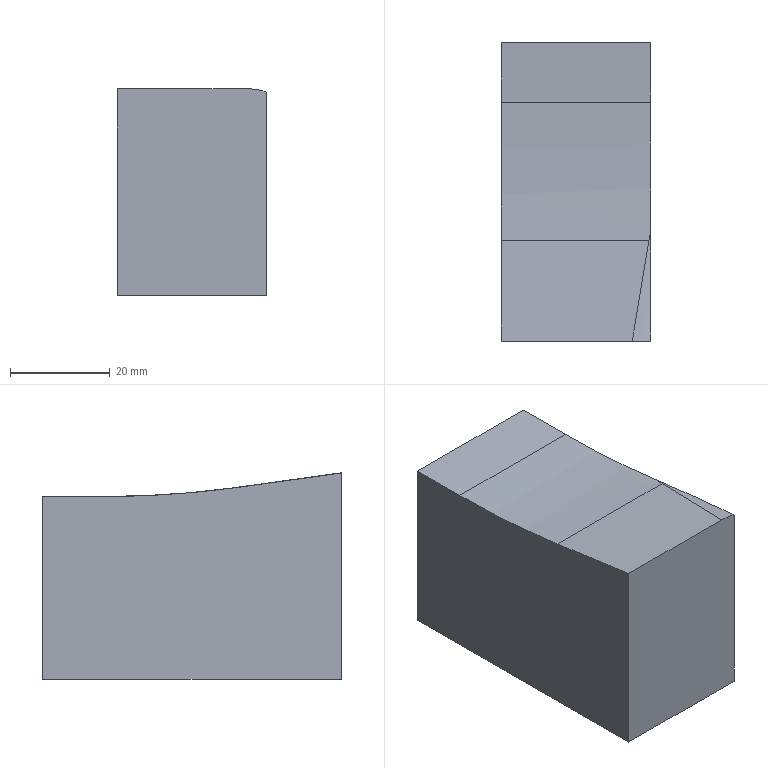Part | NX | features solid 2 | 1 solid | 10 faces | box 30 x 60 x 41.518 mm | volume 68657 mm3 | plane 5 | spline 5
STEP:
#1=CARTESIAN_POINT('',(310.,35.,31.475));
#2=VERTEX_POINT('',#1);
#3=CARTESIAN_POINT('',(336.303,35.,31.518));
#4=VERTEX_POINT('',#3);
#5=CARTESIAN_POINT('',(309.916,35.,31.475));
#6=DIRECTION('',(1.,0.,0.001631));
#7=VECTOR('',#6,1000.);
#8=LINE('',#5,#7);
#9=EDGE_CURVE('',#2,#4,#8,.T.);
#10=ORIENTED_EDGE('',*,*,#9,.F.);
#11=CARTESIAN_POINT('',(310.,35.,-10.));
#12=VERTEX_POINT('',#11);
#13=CARTESIAN_POINT('',(310.,35.,-20.));
#14=DIRECTION('',(0.,0.,1.));
#15=VECTOR('',#14,1000.);
#16=LINE('',#13,#15);
#17=EDGE_CURVE('',#12,#2,#16,.T.);
#18=ORIENTED_EDGE('',*,*,#17,.F.);
#19=CARTESIAN_POINT('',(340.,35.,-10.));
#20=VERTEX_POINT('',#19);
#21=CARTESIAN_POINT('',(310.,35.,-10.));
#22=DIRECTION('',(-1.,0.,0.));
#23=VECTOR('',#22,1000.);
#24=LINE('',#21,#23);
#25=EDGE_CURVE('',#12,#20,#24,.F.);
#26=ORIENTED_EDGE('',*,*,#25,.T.);
#27=CARTESIAN_POINT('',(340.,35.,30.835));
#28=VERTEX_POINT('',#27);
#29=CARTESIAN_POINT('',(340.,35.,-20.));
#30=DIRECTION('',(0.,0.,-1.));
#31=VECTOR('',#30,1000.);
#32=LINE('',#29,#31);
#33=EDGE_CURVE('',#20,#28,#32,.F.);
#34=ORIENTED_EDGE('',*,*,#33,.T.);
#35=CARTESIAN_POINT('',(336.303,35.,31.518));
#36=CARTESIAN_POINT('',(337.567,35.,31.52));
#37=CARTESIAN_POINT('',(338.82,35.,31.287));
#38=CARTESIAN_POINT('',(340.,35.,30.835));
#39=B_SPLINE_CURVE_WITH_KNOTS('',3,(#35,#36,#37,#38),.UNSPECIFIED.,.F.,.F.,(4,4),(0.,0.003776),.UNSPECIFIED.);
#40=EDGE_CURVE('',#4,#28,#39,.T.);
#41=ORIENTED_EDGE('',*,*,#40,.F.);
#42=EDGE_LOOP('',(#10,#18,#26,#34,#41));
#43=FACE_BOUND('',#42,.T.);
#44=CARTESIAN_POINT('',(310.,35.,-20.));
#45=DIRECTION('',(0.,1.,0.));
#46=DIRECTION('',(1.,0.,0.));
#47=AXIS2_PLACEMENT_3D('',#44,#45,#46);
#48=PLANE('',#47);
#49=ADVANCED_FACE('',(#43),#48,.F.);
#50=CARTESIAN_POINT('',(340.,95.,-10.));
#51=VERTEX_POINT('',#50);
#52=CARTESIAN_POINT('',(340.,95.,26.731));
#53=VERTEX_POINT('',#52);
#54=CARTESIAN_POINT('',(340.,95.,-20.));
#55=DIRECTION('',(0.,0.,1.));
#56=VECTOR('',#55,1000.);
#57=LINE('',#54,#56);
#58=EDGE_CURVE('',#51,#53,#57,.T.);
#59=ORIENTED_EDGE('',*,*,#58,.F.);
#60=CARTESIAN_POINT('',(310.,95.,-10.));
#61=VERTEX_POINT('',#60);
#62=CARTESIAN_POINT('',(310.,95.,-10.));
#63=DIRECTION('',(1.,0.,0.));
#64=VECTOR('',#63,1000.);
#65=LINE('',#62,#64);
#66=EDGE_CURVE('',#61,#51,#65,.T.);
#67=ORIENTED_EDGE('',*,*,#66,.F.);
#68=CARTESIAN_POINT('',(310.,95.,26.687));
#69=VERTEX_POINT('',#68);
#70=CARTESIAN_POINT('',(310.,95.,-20.));
#71=DIRECTION('',(0.,0.,1.));
#72=VECTOR('',#71,1000.);
#73=LINE('',#70,#72);
#74=EDGE_CURVE('',#61,#69,#73,.T.);
#75=ORIENTED_EDGE('',*,*,#74,.T.);
#76=CARTESIAN_POINT('',(309.932,95.,26.687));
#77=DIRECTION('',(-1.,0.,-0.001447));
#78=VECTOR('',#77,1000.);
#79=LINE('',#76,#78);
#80=EDGE_CURVE('',#53,#69,#79,.T.);
#81=ORIENTED_EDGE('',*,*,#80,.F.);
#82=EDGE_LOOP('',(#59,#67,#75,#81));
#83=FACE_BOUND('',#82,.T.);
#84=CARTESIAN_POINT('',(310.,95.,-20.));
#85=DIRECTION('',(0.,1.,0.));
#86=DIRECTION('',(1.,0.,0.));
#87=AXIS2_PLACEMENT_3D('',#84,#85,#86);
#88=PLANE('',#87);
#89=ADVANCED_FACE('',(#83),#88,.T.);
#90=ORIENTED_EDGE('',*,*,#33,.F.);
#91=CARTESIAN_POINT('',(340.,95.,-10.));
#92=DIRECTION('',(0.,-1.,0.));
#93=VECTOR('',#92,1000.);
#94=LINE('',#91,#93);
#95=EDGE_CURVE('',#51,#20,#94,.T.);
#96=ORIENTED_EDGE('',*,*,#95,.F.);
#97=ORIENTED_EDGE('',*,*,#58,.T.);
#98=CARTESIAN_POINT('',(340.,83.044,26.732));
#99=VERTEX_POINT('',#98);
#100=CARTESIAN_POINT('',(340.,83.044,26.732));
#101=CARTESIAN_POINT('',(340.,87.029,26.731));
#102=CARTESIAN_POINT('',(340.,91.015,26.731));
#103=CARTESIAN_POINT('',(340.,95.,26.731));
#104=B_SPLINE_CURVE_WITH_KNOTS('',3,(#100,#101,#102,#103),.UNSPECIFIED.,.F.,.F.,(4,4),(0.,0.01196),.UNSPECIFIED.);
#105=EDGE_CURVE('',#99,#53,#104,.T.);
#106=ORIENTED_EDGE('',*,*,#105,.F.);
#107=CARTESIAN_POINT('',(339.999,57.184,28.414));
#108=VERTEX_POINT('',#107);
#109=CARTESIAN_POINT('',(340.,57.184,28.414));
#110=CARTESIAN_POINT('',(340.,65.757,27.295));
#111=CARTESIAN_POINT('',(340.,74.397,26.733));
#112=CARTESIAN_POINT('',(340.,83.044,26.732));
#113=B_SPLINE_CURVE_WITH_KNOTS('',3,(#109,#110,#111,#112),.UNSPECIFIED.,.F.,.F.,(4,4),(0.001993,0.02793),.UNSPECIFIED.);
#114=EDGE_CURVE('',#108,#99,#113,.T.);
#115=ORIENTED_EDGE('',*,*,#114,.F.);
#116=CARTESIAN_POINT('',(340.,55.154,28.684));
#117=VERTEX_POINT('',#116);
#118=CARTESIAN_POINT('',(340.,55.154,28.684));
#119=CARTESIAN_POINT('',(340.,55.83,28.592));
#120=CARTESIAN_POINT('',(340.,56.507,28.502));
#121=CARTESIAN_POINT('',(340.,57.184,28.414));
#122=B_SPLINE_CURVE_WITH_KNOTS('',3,(#118,#119,#120,#121),.UNSPECIFIED.,.F.,.F.,(4,4),(0.,0.002048),.UNSPECIFIED.);
#123=EDGE_CURVE('',#117,#108,#122,.T.);
#124=ORIENTED_EDGE('',*,*,#123,.F.);
#125=CARTESIAN_POINT('',(340.,35.,30.835));
#126=CARTESIAN_POINT('',(340.,41.738,30.318));
#127=CARTESIAN_POINT('',(340.,48.457,29.588));
#128=CARTESIAN_POINT('',(340.,55.154,28.684));
#129=B_SPLINE_CURVE_WITH_KNOTS('',3,(#125,#126,#127,#128),.UNSPECIFIED.,.F.,.F.,(4,4),(0.,0.02027),.UNSPECIFIED.);
#130=EDGE_CURVE('',#28,#117,#129,.T.);
#131=ORIENTED_EDGE('',*,*,#130,.F.);
#132=EDGE_LOOP('',(#90,#96,#97,#106,#115,#124,#131));
#133=FACE_BOUND('',#132,.T.);
#134=CARTESIAN_POINT('',(340.,95.,-20.));
#135=DIRECTION('',(1.,0.,0.));
#136=DIRECTION('',(0.,-1.,0.));
#137=AXIS2_PLACEMENT_3D('',#134,#135,#136);
#138=PLANE('',#137);
#139=ADVANCED_FACE('',(#133),#138,.T.);
#140=ORIENTED_EDGE('',*,*,#74,.F.);
#141=CARTESIAN_POINT('',(310.,95.,-10.));
#142=DIRECTION('',(0.,1.,0.));
#143=VECTOR('',#142,1000.);
#144=LINE('',#141,#143);
#145=EDGE_CURVE('',#61,#12,#144,.F.);
#146=ORIENTED_EDGE('',*,*,#145,.T.);
#147=ORIENTED_EDGE('',*,*,#17,.T.);
#148=CARTESIAN_POINT('',(310.,55.17,28.638));
#149=VERTEX_POINT('',#148);
#150=CARTESIAN_POINT('',(310.,55.17,28.638));
#151=CARTESIAN_POINT('',(310.,48.447,29.584));
#152=CARTESIAN_POINT('',(310.,41.723,30.529));
#153=CARTESIAN_POINT('',(310.,35.,31.475));
#154=B_SPLINE_CURVE_WITH_KNOTS('',3,(#150,#151,#152,#153),.UNSPECIFIED.,.F.,.F.,(4,4),(0.,0.02037),.UNSPECIFIED.);
#155=EDGE_CURVE('',#149,#2,#154,.T.);
#156=ORIENTED_EDGE('',*,*,#155,.F.);
#157=CARTESIAN_POINT('',(310.,83.005,26.689));
#158=VERTEX_POINT('',#157);
#159=CARTESIAN_POINT('',(310.,83.005,26.689));
#160=CARTESIAN_POINT('',(310.,73.694,26.69));
#161=CARTESIAN_POINT('',(310.,64.39,27.341));
#162=CARTESIAN_POINT('',(310.,55.17,28.638));
#163=B_SPLINE_CURVE_WITH_KNOTS('',3,(#159,#160,#161,#162),.UNSPECIFIED.,.F.,.F.,(4,4),(0.,0.02793),.UNSPECIFIED.);
#164=EDGE_CURVE('',#158,#149,#163,.T.);
#165=ORIENTED_EDGE('',*,*,#164,.F.);
#166=CARTESIAN_POINT('',(310.,95.,26.687));
#167=CARTESIAN_POINT('',(310.,91.002,26.688));
#168=CARTESIAN_POINT('',(310.,87.003,26.688));
#169=CARTESIAN_POINT('',(310.,83.005,26.689));
#170=B_SPLINE_CURVE_WITH_KNOTS('',3,(#166,#167,#168,#169),.UNSPECIFIED.,.F.,.F.,(4,4),(0.,0.012),.UNSPECIFIED.);
#171=EDGE_CURVE('',#69,#158,#170,.T.);
#172=ORIENTED_EDGE('',*,*,#171,.F.);
#173=EDGE_LOOP('',(#140,#146,#147,#156,#165,#172));
#174=FACE_BOUND('',#173,.T.);
#175=CARTESIAN_POINT('',(310.,95.,-20.));
#176=DIRECTION('',(1.,0.,0.));
#177=DIRECTION('',(0.,-1.,0.));
#178=AXIS2_PLACEMENT_3D('',#175,#176,#177);
#179=PLANE('',#178);
#180=ADVANCED_FACE('',(#174),#179,.F.);
#181=ORIENTED_EDGE('',*,*,#25,.F.);
#182=ORIENTED_EDGE('',*,*,#145,.F.);
#183=ORIENTED_EDGE('',*,*,#66,.T.);
#184=ORIENTED_EDGE('',*,*,#95,.T.);
#185=EDGE_LOOP('',(#181,#182,#183,#184));
#186=FACE_BOUND('',#185,.T.);
#187=CARTESIAN_POINT('',(310.,95.,-10.));
#188=DIRECTION('',(0.,0.,1.));
#189=DIRECTION('',(1.,0.,0.));
#190=AXIS2_PLACEMENT_3D('',#187,#188,#189);
#191=PLANE('',#190);
#192=ADVANCED_FACE('',(#186),#191,.F.);
#193=ORIENTED_EDGE('',*,*,#40,.T.);
#194=ORIENTED_EDGE('',*,*,#130,.T.);
#195=CARTESIAN_POINT('',(339.665,55.209,28.681));
#196=VERTEX_POINT('',#195);
#197=CARTESIAN_POINT('',(340.,55.154,28.684));
#198=CARTESIAN_POINT('',(339.888,55.173,28.685));
#199=CARTESIAN_POINT('',(339.776,55.191,28.684));
#200=CARTESIAN_POINT('',(339.665,55.209,28.681));
#201=B_SPLINE_CURVE_WITH_KNOTS('',3,(#197,#198,#199,#200),.UNSPECIFIED.,.F.,.F.,(4,4),(0.9513,1.),.UNSPECIFIED.);
#202=EDGE_CURVE('',#117,#196,#201,.T.);
#203=ORIENTED_EDGE('',*,*,#202,.T.);
#204=CARTESIAN_POINT('',(339.665,55.209,28.681));
#205=CARTESIAN_POINT('',(338.545,48.473,29.627));
#206=CARTESIAN_POINT('',(337.424,41.736,30.572));
#207=CARTESIAN_POINT('',(336.303,35.,31.518));
#208=B_SPLINE_CURVE_WITH_KNOTS('',3,(#204,#205,#206,#207),.UNSPECIFIED.,.F.,.F.,(4,4),(0.,0.4573),.UNSPECIFIED.);
#209=EDGE_CURVE('',#196,#4,#208,.T.);
#210=ORIENTED_EDGE('',*,*,#209,.T.);
#211=EDGE_LOOP('',(#193,#194,#203,#210));
#212=FACE_BOUND('',#211,.T.);
#213=CARTESIAN_POINT('',(336.283,34.879,31.535));
#214=CARTESIAN_POINT('',(339.665,55.209,28.681));
#215=CARTESIAN_POINT('',(337.513,34.678,31.565));
#216=CARTESIAN_POINT('',(340.895,55.009,28.711));
#217=CARTESIAN_POINT('',(338.729,34.448,31.367));
#218=CARTESIAN_POINT('',(342.111,54.779,28.513));
#219=CARTESIAN_POINT('',(339.888,34.196,30.94));
#220=CARTESIAN_POINT('',(343.27,54.526,28.085));
#221=(BOUNDED_SURFACE()B_SPLINE_SURFACE(3,1,((#213,#214),(#215,#216),(#217,#218),(#219,#220)),.CYLINDRICAL_SURF.,.F.,.F.,.F.)B_SPLINE_SURFACE_WITH_KNOTS((4,4),(2,2),(0.,0.5265),(0.5399,1.),.PIECEWISE_BEZIER_KNOTS.)GEOMETRIC_REPRESENTATION_ITEM()RATIONAL_B_SPLINE_SURFACE(((1.,1.),(0.9781,0.9781),(0.9678,0.9678),(0.9689,0.9689)))REPRESENTATION_ITEM('')SURFACE());
#222=ADVANCED_FACE('',(#212),#221,.T.);
#223=ORIENTED_EDGE('',*,*,#123,.T.);
#224=CARTESIAN_POINT('',(339.998,57.185,28.414));
#225=CARTESIAN_POINT('',(339.891,56.525,28.5));
#226=CARTESIAN_POINT('',(339.78,55.867,28.589));
#227=CARTESIAN_POINT('',(339.665,55.209,28.681));
#228=B_SPLINE_CURVE_WITH_KNOTS('',3,(#224,#225,#226,#227),.UNSPECIFIED.,.F.,.F.,(4,4),(0.928,1.),.UNSPECIFIED.);
#229=EDGE_CURVE('',#108,#196,#228,.T.);
#230=ORIENTED_EDGE('',*,*,#229,.T.);
#231=ORIENTED_EDGE('',*,*,#202,.F.);
#232=EDGE_LOOP('',(#223,#230,#231));
#233=FACE_BOUND('',#232,.T.);
#234=CARTESIAN_POINT('',(340.,57.196,28.412));
#235=CARTESIAN_POINT('',(340.067,57.186,28.414));
#236=CARTESIAN_POINT('',(340.134,57.176,28.414));
#237=CARTESIAN_POINT('',(340.202,57.166,28.415));
#238=CARTESIAN_POINT('',(340.269,57.155,28.414));
#239=CARTESIAN_POINT('',(340.336,57.145,28.414));
#240=CARTESIAN_POINT('',(339.935,56.798,28.464));
#241=CARTESIAN_POINT('',(340.003,56.788,28.465));
#242=CARTESIAN_POINT('',(340.07,56.778,28.466));
#243=CARTESIAN_POINT('',(340.137,56.767,28.467));
#244=CARTESIAN_POINT('',(340.205,56.756,28.466));
#245=CARTESIAN_POINT('',(340.272,56.746,28.466));
#246=CARTESIAN_POINT('',(339.87,56.401,28.517));
#247=CARTESIAN_POINT('',(339.937,56.39,28.518));
#248=CARTESIAN_POINT('',(340.004,56.379,28.519));
#249=CARTESIAN_POINT('',(340.072,56.369,28.52));
#250=CARTESIAN_POINT('',(340.139,56.358,28.519));
#251=CARTESIAN_POINT('',(340.206,56.347,28.519));
#252=CARTESIAN_POINT('',(339.803,56.003,28.571));
#253=CARTESIAN_POINT('',(339.87,55.992,28.572));
#254=CARTESIAN_POINT('',(339.937,55.982,28.573));
#255=CARTESIAN_POINT('',(340.005,55.971,28.574));
#256=CARTESIAN_POINT('',(340.072,55.96,28.573));
#257=CARTESIAN_POINT('',(340.139,55.949,28.573));
#258=CARTESIAN_POINT('',(339.734,55.606,28.625));
#259=CARTESIAN_POINT('',(339.802,55.595,28.627));
#260=CARTESIAN_POINT('',(339.869,55.584,28.628));
#261=CARTESIAN_POINT('',(339.937,55.573,28.628));
#262=CARTESIAN_POINT('',(340.004,55.562,28.628));
#263=CARTESIAN_POINT('',(340.071,55.551,28.628));
#264=CARTESIAN_POINT('',(339.665,55.209,28.681));
#265=CARTESIAN_POINT('',(339.733,55.198,28.683));
#266=CARTESIAN_POINT('',(339.8,55.187,28.684));
#267=CARTESIAN_POINT('',(339.867,55.176,28.684));
#268=CARTESIAN_POINT('',(339.935,55.165,28.684));
#269=CARTESIAN_POINT('',(340.002,55.153,28.683));
#270=B_SPLINE_SURFACE_WITH_KNOTS('',5,5,((#234,#235,#236,#237,#238,#239),(#240,#241,#242,#243,#244,#245),(#246,#247,#248,#249,#250,#251),(#252,#253,#254,#255,#256,#257),(#258,#259,#260,#261,#262,#263),(#264,#265,#266,#267,#268,#269)),.UNSPECIFIED.,.F.,.F.,.F.,(6,6),(6,6),(0.9276,1.),(0.,0.04812),.PIECEWISE_BEZIER_KNOTS.);
#271=ADVANCED_FACE('',(#233),#270,.T.);
#272=ORIENTED_EDGE('',*,*,#105,.T.);
#273=ORIENTED_EDGE('',*,*,#80,.T.);
#274=ORIENTED_EDGE('',*,*,#171,.T.);
#275=CARTESIAN_POINT('',(340.,83.044,26.732));
#276=CARTESIAN_POINT('',(330.,83.031,26.717));
#277=CARTESIAN_POINT('',(320.,83.018,26.703));
#278=CARTESIAN_POINT('',(310.,83.005,26.689));
#279=B_SPLINE_CURVE_WITH_KNOTS('',3,(#275,#276,#277,#278),.UNSPECIFIED.,.F.,.F.,(4,4),(0.02329,0.3612),.UNSPECIFIED.);
#280=EDGE_CURVE('',#99,#158,#279,.T.);
#281=ORIENTED_EDGE('',*,*,#280,.F.);
#282=EDGE_LOOP('',(#272,#273,#274,#281));
#283=FACE_BOUND('',#282,.T.);
#284=CARTESIAN_POINT('',(309.82,83.005,26.688));
#285=CARTESIAN_POINT('',(340.196,83.044,26.732));
#286=CARTESIAN_POINT('',(309.804,95.072,26.687));
#287=CARTESIAN_POINT('',(340.18,95.111,26.731));
#288=B_SPLINE_SURFACE_WITH_KNOTS('',1,1,((#284,#285),(#286,#287)),.PLANE_SURF.,.F.,.F.,.F.,(2,2),(2,2),(0.,0.1247),(0.5749,0.8807),.PIECEWISE_BEZIER_KNOTS.);
#289=ADVANCED_FACE('',(#283),#288,.F.);
#290=ORIENTED_EDGE('',*,*,#114,.T.);
#291=ORIENTED_EDGE('',*,*,#280,.T.);
#292=ORIENTED_EDGE('',*,*,#164,.T.);
#293=CARTESIAN_POINT('',(339.665,55.209,28.681));
#294=CARTESIAN_POINT('',(329.777,55.196,28.667));
#295=CARTESIAN_POINT('',(319.888,55.183,28.652));
#296=CARTESIAN_POINT('',(310.,55.17,28.638));
#297=B_SPLINE_CURVE_WITH_KNOTS('',3,(#293,#294,#295,#296),.UNSPECIFIED.,.F.,.F.,(4,4),(0.,0.2337),.UNSPECIFIED.);
#298=EDGE_CURVE('',#196,#149,#297,.T.);
#299=ORIENTED_EDGE('',*,*,#298,.F.);
#300=ORIENTED_EDGE('',*,*,#229,.F.);
#301=EDGE_LOOP('',(#290,#291,#292,#299,#300));
#302=FACE_BOUND('',#301,.T.);
#303=CARTESIAN_POINT('',(309.82,55.17,28.638));
#304=CARTESIAN_POINT('',(340.214,55.21,28.682));
#305=CARTESIAN_POINT('',(309.81,64.395,27.34));
#306=CARTESIAN_POINT('',(340.204,64.435,27.384));
#307=CARTESIAN_POINT('',(309.798,73.689,26.689));
#308=CARTESIAN_POINT('',(340.192,73.728,26.733));
#309=CARTESIAN_POINT('',(309.786,83.005,26.688));
#310=CARTESIAN_POINT('',(340.18,83.044,26.732));
#311=(BOUNDED_SURFACE()B_SPLINE_SURFACE(3,1,((#303,#304),(#305,#306),(#307,#308),(#309,#310)),.CYLINDRICAL_SURF.,.F.,.F.,.F.)B_SPLINE_SURFACE_WITH_KNOTS((4,4),(2,2),(0.,1.),(0.7475,0.9797),.PIECEWISE_BEZIER_KNOTS.)GEOMETRIC_REPRESENTATION_ITEM()RATIONAL_B_SPLINE_SURFACE(((1.,1.),(0.9984,0.9984),(0.9984,0.9984),(1.,1.)))REPRESENTATION_ITEM('')SURFACE());
#312=ADVANCED_FACE('',(#302),#311,.F.);
#313=ORIENTED_EDGE('',*,*,#9,.T.);
#314=ORIENTED_EDGE('',*,*,#209,.F.);
#315=ORIENTED_EDGE('',*,*,#298,.T.);
#316=ORIENTED_EDGE('',*,*,#155,.T.);
#317=EDGE_LOOP('',(#313,#314,#315,#316));
#318=FACE_BOUND('',#317,.T.);
#319=CARTESIAN_POINT('',(309.8,55.17,28.638));
#320=CARTESIAN_POINT('',(339.843,55.209,28.681));
#321=CARTESIAN_POINT('',(309.822,34.844,31.497));
#322=CARTESIAN_POINT('',(339.866,34.883,31.54));
#323=B_SPLINE_SURFACE_WITH_KNOTS('',1,1,((#319,#320),(#321,#322)),.PLANE_SURF.,.F.,.F.,.F.,(2,2),(2,2),(0.,0.1645),(0.8363,0.995),.PIECEWISE_BEZIER_KNOTS.);
#324=ADVANCED_FACE('',(#318),#323,.T.);
#325=CLOSED_SHELL('',(#49,#89,#139,#180,#192,#222,#271,#289,#312,#324));
#326=MANIFOLD_SOLID_BREP('',#325);
#327=(LENGTH_UNIT()NAMED_UNIT(*)SI_UNIT(.MILLI.,.METRE.));
#328=UNCERTAINTY_MEASURE_WITH_UNIT(LENGTH_MEASURE(0.05316),#327,'','');
#329=(NAMED_UNIT(*)PLANE_ANGLE_UNIT()SI_UNIT($,.RADIAN.));
#330=(NAMED_UNIT(*)SI_UNIT($,.STERADIAN.)SOLID_ANGLE_UNIT());
#331=(GEOMETRIC_REPRESENTATION_CONTEXT(3)GLOBAL_UNCERTAINTY_ASSIGNED_CONTEXT((#328))GLOBAL_UNIT_ASSIGNED_CONTEXT((#327,#329,#330))REPRESENTATION_CONTEXT('',''));
#332=ADVANCED_BREP_SHAPE_REPRESENTATION('',(#326),#331);